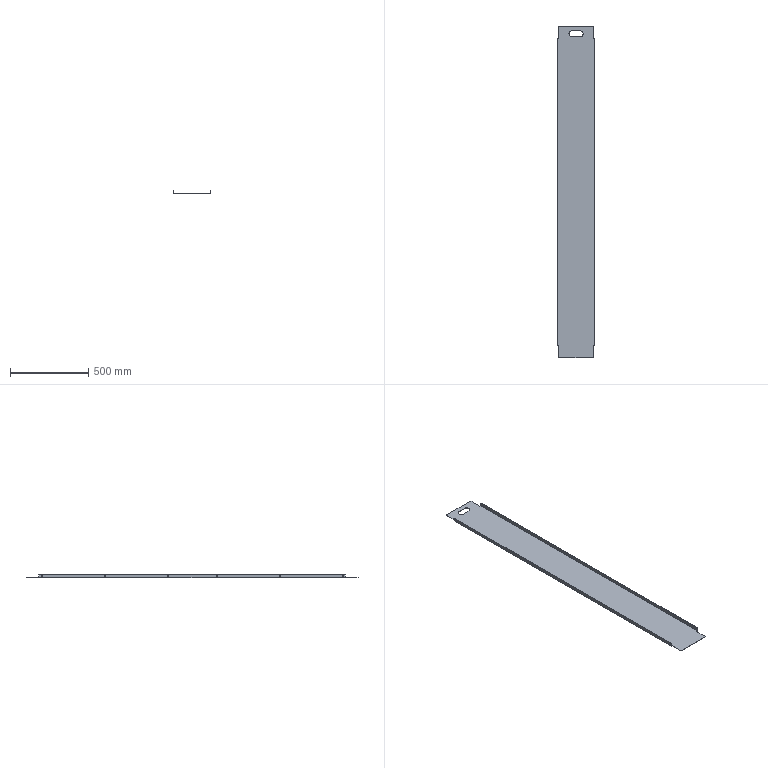Part | SolidWorks | features Chamfer 2, ICE 2, Cut 1, FlatPattern 1, SMBaseFlange 1, SheetMetal 1 | 1 solid | 65 faces | box 240 x 2116 x 23 mm | volume 875220 mm3 | plane 34 | cylinder 31 | commonest cylinder face diameters 6.2 x24 40 x3 0.4 x2 3.4 x2